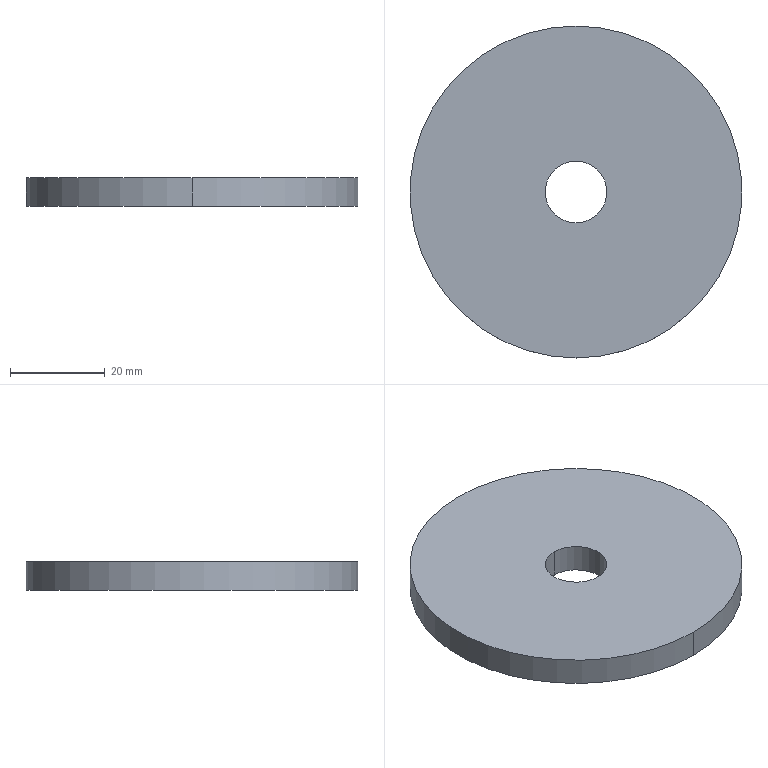Part | STEP file | 1 solid | 6 faces | box 70 x 70 x 6 mm | volume 22294 mm3 | cylinder 4 | plane 2 | commonest cylinder face diameters 13 x2 70 x2
STEP:
#1=CARTESIAN_POINT('',(0.,0.,0.));
#2=DIRECTION('',(0.,0.,1.));
#3=DIRECTION('',(1.,0.,0.));
#4=AXIS2_PLACEMENT_3D('',#1,#2,#3);
#5=CARTESIAN_POINT('',(0.,6.5,0.));
#6=VERTEX_POINT('',#5);
#7=CARTESIAN_POINT('',(0.,-6.5,0.));
#8=VERTEX_POINT('',#7);
#9=CARTESIAN_POINT('',(0.,0.,0.));
#10=DIRECTION('',(0.,0.,1.));
#11=DIRECTION('',(0.,1.,0.));
#12=AXIS2_PLACEMENT_3D('',#9,#10,#11);
#13=CIRCLE('',#12,6.5);
#14=CARTESIAN_POINT('',(0.,0.,0.));
#15=DIRECTION('',(0.,0.,1.));
#16=DIRECTION('',(0.,-1.,0.));
#17=AXIS2_PLACEMENT_3D('',#14,#15,#16);
#18=PLANE('',#17);
#19=CARTESIAN_POINT('',(0.,0.));
#20=DIRECTION('',(-1.,0.));
#21=AXIS2_PLACEMENT_2D('',#19,#20);
#22=CIRCLE('',#21,6.5);
#23=(GEOMETRIC_REPRESENTATION_CONTEXT(2)PARAMETRIC_REPRESENTATION_CONTEXT()REPRESENTATION_CONTEXT('',''));
#24=DEFINITIONAL_REPRESENTATION('',(#22),#23);
#25=PCURVE('',#18,#24);
#26=CARTESIAN_POINT('',(0.,0.,6.));
#27=DIRECTION('',(0.,0.,-1.));
#28=DIRECTION('',(0.,1.,0.));
#29=AXIS2_PLACEMENT_3D('',#26,#27,#28);
#30=CYLINDRICAL_SURFACE('',#29,6.5);
#31=CARTESIAN_POINT('',(6.283,6.));
#32=DIRECTION('',(-1.,0.));
#33=VECTOR('',#32,1.);
#34=LINE('',#31,#33);
#35=(GEOMETRIC_REPRESENTATION_CONTEXT(2)PARAMETRIC_REPRESENTATION_CONTEXT()REPRESENTATION_CONTEXT('',''));
#36=DEFINITIONAL_REPRESENTATION('',(#34),#35);
#37=PCURVE('',#30,#36);
#38=SURFACE_CURVE('',#13,(#25,#37),.PCURVE_S1.);
#39=EDGE_CURVE('',#6,#8,#38,.T.);
#40=ORIENTED_EDGE('',*,*,#39,.T.);
#41=CARTESIAN_POINT('',(0.,0.,0.));
#42=DIRECTION('',(0.,0.,1.));
#43=DIRECTION('',(0.,1.,0.));
#44=AXIS2_PLACEMENT_3D('',#41,#42,#43);
#45=CIRCLE('',#44,6.5);
#46=CARTESIAN_POINT('',(0.,0.));
#47=DIRECTION('',(-1.,0.));
#48=AXIS2_PLACEMENT_2D('',#46,#47);
#49=CIRCLE('',#48,6.5);
#50=(GEOMETRIC_REPRESENTATION_CONTEXT(2)PARAMETRIC_REPRESENTATION_CONTEXT()REPRESENTATION_CONTEXT('',''));
#51=DEFINITIONAL_REPRESENTATION('',(#49),#50);
#52=PCURVE('',#18,#51);
#53=CARTESIAN_POINT('',(0.,0.,6.));
#54=DIRECTION('',(0.,0.,-1.));
#55=DIRECTION('',(0.,1.,0.));
#56=AXIS2_PLACEMENT_3D('',#53,#54,#55);
#57=CYLINDRICAL_SURFACE('',#56,6.5);
#58=CARTESIAN_POINT('',(6.283,6.));
#59=DIRECTION('',(-1.,0.));
#60=VECTOR('',#59,1.);
#61=LINE('',#58,#60);
#62=(GEOMETRIC_REPRESENTATION_CONTEXT(2)PARAMETRIC_REPRESENTATION_CONTEXT()REPRESENTATION_CONTEXT('',''));
#63=DEFINITIONAL_REPRESENTATION('',(#61),#62);
#64=PCURVE('',#57,#63);
#65=SURFACE_CURVE('',#45,(#52,#64),.PCURVE_S1.);
#66=EDGE_CURVE('',#8,#6,#65,.T.);
#67=ORIENTED_EDGE('',*,*,#66,.T.);
#68=EDGE_LOOP('',(#40,#67));
#69=FACE_BOUND('',#68,.T.);
#70=CARTESIAN_POINT('',(0.,35.,0.));
#71=VERTEX_POINT('',#70);
#72=CARTESIAN_POINT('',(0.,-35.,0.));
#73=VERTEX_POINT('',#72);
#74=CARTESIAN_POINT('',(0.,0.,0.));
#75=DIRECTION('',(0.,0.,1.));
#76=DIRECTION('',(0.,1.,0.));
#77=AXIS2_PLACEMENT_3D('',#74,#75,#76);
#78=CIRCLE('',#77,35.);
#79=CARTESIAN_POINT('',(0.,0.));
#80=DIRECTION('',(-1.,0.));
#81=AXIS2_PLACEMENT_2D('',#79,#80);
#82=CIRCLE('',#81,35.);
#83=(GEOMETRIC_REPRESENTATION_CONTEXT(2)PARAMETRIC_REPRESENTATION_CONTEXT()REPRESENTATION_CONTEXT('',''));
#84=DEFINITIONAL_REPRESENTATION('',(#82),#83);
#85=PCURVE('',#18,#84);
#86=CARTESIAN_POINT('',(0.,0.,6.));
#87=DIRECTION('',(0.,0.,-1.));
#88=DIRECTION('',(0.,1.,0.));
#89=AXIS2_PLACEMENT_3D('',#86,#87,#88);
#90=CYLINDRICAL_SURFACE('',#89,35.);
#91=CARTESIAN_POINT('',(6.283,6.));
#92=DIRECTION('',(-1.,0.));
#93=VECTOR('',#92,1.);
#94=LINE('',#91,#93);
#95=(GEOMETRIC_REPRESENTATION_CONTEXT(2)PARAMETRIC_REPRESENTATION_CONTEXT()REPRESENTATION_CONTEXT('',''));
#96=DEFINITIONAL_REPRESENTATION('',(#94),#95);
#97=PCURVE('',#90,#96);
#98=SURFACE_CURVE('',#78,(#85,#97),.PCURVE_S1.);
#99=EDGE_CURVE('',#71,#73,#98,.T.);
#100=ORIENTED_EDGE('',*,*,#99,.F.);
#101=CARTESIAN_POINT('',(0.,0.,0.));
#102=DIRECTION('',(0.,0.,1.));
#103=DIRECTION('',(0.,1.,0.));
#104=AXIS2_PLACEMENT_3D('',#101,#102,#103);
#105=CIRCLE('',#104,35.);
#106=CARTESIAN_POINT('',(0.,0.));
#107=DIRECTION('',(-1.,0.));
#108=AXIS2_PLACEMENT_2D('',#106,#107);
#109=CIRCLE('',#108,35.);
#110=(GEOMETRIC_REPRESENTATION_CONTEXT(2)PARAMETRIC_REPRESENTATION_CONTEXT()REPRESENTATION_CONTEXT('',''));
#111=DEFINITIONAL_REPRESENTATION('',(#109),#110);
#112=PCURVE('',#18,#111);
#113=CARTESIAN_POINT('',(0.,0.,6.));
#114=DIRECTION('',(0.,0.,-1.));
#115=DIRECTION('',(0.,1.,0.));
#116=AXIS2_PLACEMENT_3D('',#113,#114,#115);
#117=CYLINDRICAL_SURFACE('',#116,35.);
#118=CARTESIAN_POINT('',(6.283,6.));
#119=DIRECTION('',(-1.,0.));
#120=VECTOR('',#119,1.);
#121=LINE('',#118,#120);
#122=(GEOMETRIC_REPRESENTATION_CONTEXT(2)PARAMETRIC_REPRESENTATION_CONTEXT()REPRESENTATION_CONTEXT('',''));
#123=DEFINITIONAL_REPRESENTATION('',(#121),#122);
#124=PCURVE('',#117,#123);
#125=SURFACE_CURVE('',#105,(#112,#124),.PCURVE_S1.);
#126=EDGE_CURVE('',#73,#71,#125,.T.);
#127=ORIENTED_EDGE('',*,*,#126,.F.);
#128=EDGE_LOOP('',(#100,#127));
#129=FACE_BOUND('',#128,.T.);
#130=ADVANCED_FACE('',(#69,#129),#18,.F.);
#131=CARTESIAN_POINT('',(0.,-35.,6.));
#132=VERTEX_POINT('',#131);
#133=CARTESIAN_POINT('',(0.,-35.,6.));
#134=DIRECTION('',(0.,0.,-1.));
#135=VECTOR('',#134,1.);
#136=LINE('',#133,#135);
#137=CARTESIAN_POINT('',(3.142,0.));
#138=DIRECTION('',(0.,1.));
#139=VECTOR('',#138,1.);
#140=LINE('',#137,#139);
#141=(GEOMETRIC_REPRESENTATION_CONTEXT(2)PARAMETRIC_REPRESENTATION_CONTEXT()REPRESENTATION_CONTEXT('',''));
#142=DEFINITIONAL_REPRESENTATION('',(#140),#141);
#143=PCURVE('',#90,#142);
#144=CARTESIAN_POINT('',(3.142,0.));
#145=DIRECTION('',(0.,1.));
#146=VECTOR('',#145,1.);
#147=LINE('',#144,#146);
#148=(GEOMETRIC_REPRESENTATION_CONTEXT(2)PARAMETRIC_REPRESENTATION_CONTEXT()REPRESENTATION_CONTEXT('',''));
#149=DEFINITIONAL_REPRESENTATION('',(#147),#148);
#150=PCURVE('',#117,#149);
#151=SURFACE_CURVE('',#136,(#143,#150),.PCURVE_S1.);
#152=EDGE_CURVE('',#132,#73,#151,.T.);
#153=ORIENTED_EDGE('',*,*,#152,.F.);
#154=CARTESIAN_POINT('',(0.,35.,6.));
#155=VERTEX_POINT('',#154);
#156=CARTESIAN_POINT('',(0.,0.,6.));
#157=DIRECTION('',(0.,0.,1.));
#158=DIRECTION('',(0.,1.,0.));
#159=AXIS2_PLACEMENT_3D('',#156,#157,#158);
#160=CIRCLE('',#159,35.);
#161=CARTESIAN_POINT('',(6.283,0.));
#162=DIRECTION('',(-1.,0.));
#163=VECTOR('',#162,1.);
#164=LINE('',#161,#163);
#165=(GEOMETRIC_REPRESENTATION_CONTEXT(2)PARAMETRIC_REPRESENTATION_CONTEXT()REPRESENTATION_CONTEXT('',''));
#166=DEFINITIONAL_REPRESENTATION('',(#164),#165);
#167=PCURVE('',#90,#166);
#168=CARTESIAN_POINT('',(0.,0.,6.));
#169=DIRECTION('',(0.,0.,1.));
#170=DIRECTION('',(0.,-1.,0.));
#171=AXIS2_PLACEMENT_3D('',#168,#169,#170);
#172=PLANE('',#171);
#173=CARTESIAN_POINT('',(0.,0.));
#174=DIRECTION('',(-1.,0.));
#175=AXIS2_PLACEMENT_2D('',#173,#174);
#176=CIRCLE('',#175,35.);
#177=(GEOMETRIC_REPRESENTATION_CONTEXT(2)PARAMETRIC_REPRESENTATION_CONTEXT()REPRESENTATION_CONTEXT('',''));
#178=DEFINITIONAL_REPRESENTATION('',(#176),#177);
#179=PCURVE('',#172,#178);
#180=SURFACE_CURVE('',#160,(#167,#179),.PCURVE_S1.);
#181=EDGE_CURVE('',#155,#132,#180,.T.);
#182=ORIENTED_EDGE('',*,*,#181,.F.);
#183=CARTESIAN_POINT('',(0.,35.,6.));
#184=DIRECTION('',(0.,0.,-1.));
#185=VECTOR('',#184,1.);
#186=LINE('',#183,#185);
#187=CARTESIAN_POINT('',(6.283,0.));
#188=DIRECTION('',(0.,1.));
#189=VECTOR('',#188,1.);
#190=LINE('',#187,#189);
#191=(GEOMETRIC_REPRESENTATION_CONTEXT(2)PARAMETRIC_REPRESENTATION_CONTEXT()REPRESENTATION_CONTEXT('',''));
#192=DEFINITIONAL_REPRESENTATION('',(#190),#191);
#193=PCURVE('',#90,#192);
#194=CARTESIAN_POINT('',(0.,0.));
#195=DIRECTION('',(0.,1.));
#196=VECTOR('',#195,1.);
#197=LINE('',#194,#196);
#198=(GEOMETRIC_REPRESENTATION_CONTEXT(2)PARAMETRIC_REPRESENTATION_CONTEXT()REPRESENTATION_CONTEXT('',''));
#199=DEFINITIONAL_REPRESENTATION('',(#197),#198);
#200=PCURVE('',#117,#199);
#201=SURFACE_CURVE('',#186,(#193,#200),.PCURVE_S1.);
#202=EDGE_CURVE('',#155,#71,#201,.T.);
#203=ORIENTED_EDGE('',*,*,#202,.T.);
#204=ORIENTED_EDGE('',*,*,#99,.T.);
#205=EDGE_LOOP('',(#153,#182,#203,#204));
#206=FACE_BOUND('',#205,.T.);
#207=ADVANCED_FACE('',(#206),#90,.T.);
#208=ORIENTED_EDGE('',*,*,#66,.T.);
#209=CARTESIAN_POINT('',(0.,6.5,6.));
#210=VERTEX_POINT('',#209);
#211=CARTESIAN_POINT('',(0.,6.5,6.));
#212=DIRECTION('',(0.,0.,-1.));
#213=VECTOR('',#212,1.);
#214=LINE('',#211,#213);
#215=CARTESIAN_POINT('',(0.,0.));
#216=DIRECTION('',(0.,1.));
#217=VECTOR('',#216,1.);
#218=LINE('',#215,#217);
#219=(GEOMETRIC_REPRESENTATION_CONTEXT(2)PARAMETRIC_REPRESENTATION_CONTEXT()REPRESENTATION_CONTEXT('',''));
#220=DEFINITIONAL_REPRESENTATION('',(#218),#219);
#221=PCURVE('',#57,#220);
#222=CARTESIAN_POINT('',(6.283,0.));
#223=DIRECTION('',(0.,1.));
#224=VECTOR('',#223,1.);
#225=LINE('',#222,#224);
#226=(GEOMETRIC_REPRESENTATION_CONTEXT(2)PARAMETRIC_REPRESENTATION_CONTEXT()REPRESENTATION_CONTEXT('',''));
#227=DEFINITIONAL_REPRESENTATION('',(#225),#226);
#228=PCURVE('',#30,#227);
#229=SURFACE_CURVE('',#214,(#221,#228),.PCURVE_S1.);
#230=EDGE_CURVE('',#210,#6,#229,.T.);
#231=ORIENTED_EDGE('',*,*,#230,.F.);
#232=CARTESIAN_POINT('',(0.,-6.5,6.));
#233=VERTEX_POINT('',#232);
#234=CARTESIAN_POINT('',(0.,0.,6.));
#235=DIRECTION('',(0.,0.,-1.));
#236=DIRECTION('',(0.,1.,0.));
#237=AXIS2_PLACEMENT_3D('',#234,#235,#236);
#238=CIRCLE('',#237,6.5);
#239=CARTESIAN_POINT('',(0.,0.));
#240=DIRECTION('',(1.,0.));
#241=VECTOR('',#240,1.);
#242=LINE('',#239,#241);
#243=(GEOMETRIC_REPRESENTATION_CONTEXT(2)PARAMETRIC_REPRESENTATION_CONTEXT()REPRESENTATION_CONTEXT('',''));
#244=DEFINITIONAL_REPRESENTATION('',(#242),#243);
#245=PCURVE('',#57,#244);
#246=CARTESIAN_POINT('',(-6.5,0.));
#247=CARTESIAN_POINT('',(-6.5,11.258));
#248=CARTESIAN_POINT('',(3.25,5.629));
#249=CARTESIAN_POINT('',(13.,0.));
#250=CARTESIAN_POINT('',(3.25,-5.629));
#251=CARTESIAN_POINT('',(-6.5,-11.258));
#252=CARTESIAN_POINT('',(-6.5,0.));
#253=(BOUNDED_CURVE()B_SPLINE_CURVE(2,(#246,#247,#248,#249,#250,#251,#252),.UNSPECIFIED.,.T.,.F.)B_SPLINE_CURVE_WITH_KNOTS((1,2,2,2,2,1),(-2.094,0.,2.094,4.189,6.283,8.378),.UNSPECIFIED.)CURVE()GEOMETRIC_REPRESENTATION_ITEM()RATIONAL_B_SPLINE_CURVE((1.,0.5,1.,0.5,1.,0.5,1.))REPRESENTATION_ITEM(''));
#254=(GEOMETRIC_REPRESENTATION_CONTEXT(2)PARAMETRIC_REPRESENTATION_CONTEXT()REPRESENTATION_CONTEXT('',''));
#255=DEFINITIONAL_REPRESENTATION('',(#253),#254);
#256=PCURVE('',#172,#255);
#257=SURFACE_CURVE('',#238,(#245,#256),.PCURVE_S1.);
#258=EDGE_CURVE('',#210,#233,#257,.T.);
#259=ORIENTED_EDGE('',*,*,#258,.T.);
#260=CARTESIAN_POINT('',(0.,-6.5,6.));
#261=DIRECTION('',(0.,0.,-1.));
#262=VECTOR('',#261,1.);
#263=LINE('',#260,#262);
#264=CARTESIAN_POINT('',(3.142,0.));
#265=DIRECTION('',(0.,1.));
#266=VECTOR('',#265,1.);
#267=LINE('',#264,#266);
#268=(GEOMETRIC_REPRESENTATION_CONTEXT(2)PARAMETRIC_REPRESENTATION_CONTEXT()REPRESENTATION_CONTEXT('',''));
#269=DEFINITIONAL_REPRESENTATION('',(#267),#268);
#270=PCURVE('',#57,#269);
#271=CARTESIAN_POINT('',(3.142,0.));
#272=DIRECTION('',(0.,1.));
#273=VECTOR('',#272,1.);
#274=LINE('',#271,#273);
#275=(GEOMETRIC_REPRESENTATION_CONTEXT(2)PARAMETRIC_REPRESENTATION_CONTEXT()REPRESENTATION_CONTEXT('',''));
#276=DEFINITIONAL_REPRESENTATION('',(#274),#275);
#277=PCURVE('',#30,#276);
#278=SURFACE_CURVE('',#263,(#270,#277),.PCURVE_S1.);
#279=EDGE_CURVE('',#233,#8,#278,.T.);
#280=ORIENTED_EDGE('',*,*,#279,.T.);
#281=EDGE_LOOP('',(#208,#231,#259,#280));
#282=FACE_BOUND('',#281,.F.);
#283=ADVANCED_FACE('',(#282),#57,.F.);
#284=ORIENTED_EDGE('',*,*,#258,.T.);
#285=CARTESIAN_POINT('',(0.,0.,6.));
#286=DIRECTION('',(0.,0.,-1.));
#287=DIRECTION('',(0.,1.,0.));
#288=AXIS2_PLACEMENT_3D('',#285,#286,#287);
#289=CIRCLE('',#288,6.5);
#290=CARTESIAN_POINT('',(-6.5,0.));
#291=CARTESIAN_POINT('',(-6.5,11.258));
#292=CARTESIAN_POINT('',(3.25,5.629));
#293=CARTESIAN_POINT('',(13.,0.));
#294=CARTESIAN_POINT('',(3.25,-5.629));
#295=CARTESIAN_POINT('',(-6.5,-11.258));
#296=CARTESIAN_POINT('',(-6.5,0.));
#297=(BOUNDED_CURVE()B_SPLINE_CURVE(2,(#290,#291,#292,#293,#294,#295,#296),.UNSPECIFIED.,.T.,.F.)B_SPLINE_CURVE_WITH_KNOTS((1,2,2,2,2,1),(-2.094,0.,2.094,4.189,6.283,8.378),.UNSPECIFIED.)CURVE()GEOMETRIC_REPRESENTATION_ITEM()RATIONAL_B_SPLINE_CURVE((1.,0.5,1.,0.5,1.,0.5,1.))REPRESENTATION_ITEM(''));
#298=(GEOMETRIC_REPRESENTATION_CONTEXT(2)PARAMETRIC_REPRESENTATION_CONTEXT()REPRESENTATION_CONTEXT('',''));
#299=DEFINITIONAL_REPRESENTATION('',(#297),#298);
#300=PCURVE('',#172,#299);
#301=CARTESIAN_POINT('',(0.,0.));
#302=DIRECTION('',(1.,0.));
#303=VECTOR('',#302,1.);
#304=LINE('',#301,#303);
#305=(GEOMETRIC_REPRESENTATION_CONTEXT(2)PARAMETRIC_REPRESENTATION_CONTEXT()REPRESENTATION_CONTEXT('',''));
#306=DEFINITIONAL_REPRESENTATION('',(#304),#305);
#307=PCURVE('',#30,#306);
#308=SURFACE_CURVE('',#289,(#300,#307),.PCURVE_S1.);
#309=EDGE_CURVE('',#233,#210,#308,.T.);
#310=ORIENTED_EDGE('',*,*,#309,.T.);
#311=EDGE_LOOP('',(#284,#310));
#312=FACE_BOUND('',#311,.T.);
#313=ORIENTED_EDGE('',*,*,#181,.T.);
#314=CARTESIAN_POINT('',(0.,0.,6.));
#315=DIRECTION('',(0.,0.,1.));
#316=DIRECTION('',(0.,1.,0.));
#317=AXIS2_PLACEMENT_3D('',#314,#315,#316);
#318=CIRCLE('',#317,35.);
#319=CARTESIAN_POINT('',(0.,0.));
#320=DIRECTION('',(-1.,0.));
#321=AXIS2_PLACEMENT_2D('',#319,#320);
#322=CIRCLE('',#321,35.);
#323=(GEOMETRIC_REPRESENTATION_CONTEXT(2)PARAMETRIC_REPRESENTATION_CONTEXT()REPRESENTATION_CONTEXT('',''));
#324=DEFINITIONAL_REPRESENTATION('',(#322),#323);
#325=PCURVE('',#172,#324);
#326=CARTESIAN_POINT('',(6.283,0.));
#327=DIRECTION('',(-1.,0.));
#328=VECTOR('',#327,1.);
#329=LINE('',#326,#328);
#330=(GEOMETRIC_REPRESENTATION_CONTEXT(2)PARAMETRIC_REPRESENTATION_CONTEXT()REPRESENTATION_CONTEXT('',''));
#331=DEFINITIONAL_REPRESENTATION('',(#329),#330);
#332=PCURVE('',#117,#331);
#333=SURFACE_CURVE('',#318,(#325,#332),.PCURVE_S1.);
#334=EDGE_CURVE('',#132,#155,#333,.T.);
#335=ORIENTED_EDGE('',*,*,#334,.T.);
#336=EDGE_LOOP('',(#313,#335));
#337=FACE_BOUND('',#336,.T.);
#338=ADVANCED_FACE('',(#312,#337),#172,.T.);
#339=ORIENTED_EDGE('',*,*,#334,.F.);
#340=ORIENTED_EDGE('',*,*,#152,.T.);
#341=ORIENTED_EDGE('',*,*,#126,.T.);
#342=ORIENTED_EDGE('',*,*,#202,.F.);
#343=EDGE_LOOP('',(#339,#340,#341,#342));
#344=FACE_BOUND('',#343,.T.);
#345=ADVANCED_FACE('',(#344),#117,.T.);
#346=ORIENTED_EDGE('',*,*,#230,.T.);
#347=ORIENTED_EDGE('',*,*,#39,.T.);
#348=ORIENTED_EDGE('',*,*,#279,.F.);
#349=ORIENTED_EDGE('',*,*,#309,.T.);
#350=EDGE_LOOP('',(#346,#347,#348,#349));
#351=FACE_BOUND('',#350,.F.);
#352=ADVANCED_FACE('',(#351),#30,.F.);
#353=CLOSED_SHELL('',(#130,#207,#283,#338,#345,#352));
#354=MANIFOLD_SOLID_BREP('',#353);
#355=(LENGTH_UNIT()NAMED_UNIT(*)SI_UNIT(.MILLI.,.METRE.));
#356=UNCERTAINTY_MEASURE_WITH_UNIT(LENGTH_MEASURE(0.0000001),#355,'','');
#357=(NAMED_UNIT(*)PLANE_ANGLE_UNIT()SI_UNIT($,.RADIAN.));
#358=(NAMED_UNIT(*)SI_UNIT($,.STERADIAN.)SOLID_ANGLE_UNIT());
#359=(GEOMETRIC_REPRESENTATION_CONTEXT(3)GLOBAL_UNCERTAINTY_ASSIGNED_CONTEXT((#356))GLOBAL_UNIT_ASSIGNED_CONTEXT((#355,#357,#358))REPRESENTATION_CONTEXT('',''));
#360=ADVANCED_BREP_SHAPE_REPRESENTATION('',(#4,#354),#359);